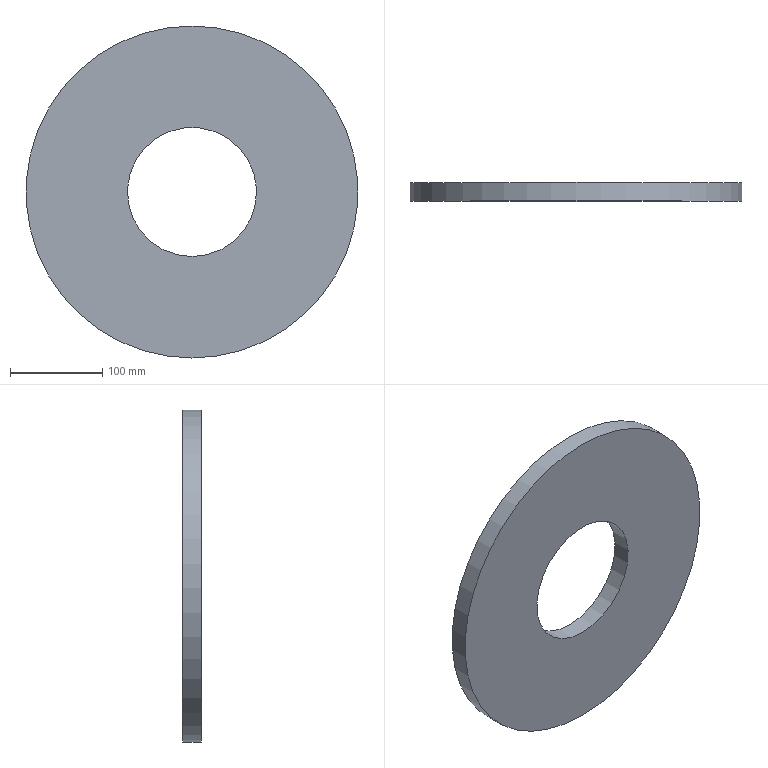Part | STEP file | 冲床-300配套压波_id730_x_t | 1 solid | 4 faces | box 360 x 20 x 360 mm | volume 1727876 mm3 | plane 2 | cylinder 2 | commonest cylinder face diameters 140 x1 360 x1
STEP:
#1=CARTESIAN_POINT('',(2195.,-10.,-275.));
#2=VERTEX_POINT('',#1);
#3=CARTESIAN_POINT('',(2195.,-10.,-205.));
#4=DIRECTION('',(0.,-1.,0.));
#5=DIRECTION('',(0.,0.,-1.));
#6=AXIS2_PLACEMENT_3D('',#3,#4,#5);
#7=CIRCLE('',#6,70.);
#8=EDGE_CURVE('',#2,#2,#7,.T.);
#9=ORIENTED_EDGE('',*,*,#8,.F.);
#10=EDGE_LOOP('',(#9));
#11=FACE_BOUND('',#10,.T.);
#12=CARTESIAN_POINT('',(2195.,-10.,-385.));
#13=VERTEX_POINT('',#12);
#14=CARTESIAN_POINT('',(2195.,-10.,-205.));
#15=DIRECTION('',(0.,-1.,0.));
#16=DIRECTION('',(0.,0.,-1.));
#17=AXIS2_PLACEMENT_3D('',#14,#15,#16);
#18=CIRCLE('',#17,180.);
#19=EDGE_CURVE('',#13,#13,#18,.T.);
#20=ORIENTED_EDGE('',*,*,#19,.T.);
#21=EDGE_LOOP('',(#20));
#22=FACE_BOUND('',#21,.T.);
#23=CARTESIAN_POINT('',(432.953,-10.,916.258));
#24=DIRECTION('',(0.,-1.,0.));
#25=DIRECTION('',(-0.5361,0.,-0.8442));
#26=AXIS2_PLACEMENT_3D('',#23,#24,#25);
#27=PLANE('',#26);
#28=ADVANCED_FACE('',(#11,#22),#27,.T.);
#29=CARTESIAN_POINT('',(2195.,10.,-275.));
#30=VERTEX_POINT('',#29);
#31=CARTESIAN_POINT('',(2195.,10.,-205.));
#32=DIRECTION('',(0.,-1.,0.));
#33=DIRECTION('',(0.,0.,-1.));
#34=AXIS2_PLACEMENT_3D('',#31,#32,#33);
#35=CIRCLE('',#34,70.);
#36=EDGE_CURVE('',#30,#30,#35,.T.);
#37=ORIENTED_EDGE('',*,*,#36,.T.);
#38=EDGE_LOOP('',(#37));
#39=FACE_BOUND('',#38,.T.);
#40=CARTESIAN_POINT('',(2195.,10.,-385.));
#41=VERTEX_POINT('',#40);
#42=CARTESIAN_POINT('',(2195.,10.,-205.));
#43=DIRECTION('',(0.,-1.,0.));
#44=DIRECTION('',(0.,0.,-1.));
#45=AXIS2_PLACEMENT_3D('',#42,#43,#44);
#46=CIRCLE('',#45,180.);
#47=EDGE_CURVE('',#41,#41,#46,.T.);
#48=ORIENTED_EDGE('',*,*,#47,.F.);
#49=EDGE_LOOP('',(#48));
#50=FACE_BOUND('',#49,.T.);
#51=CARTESIAN_POINT('',(432.953,10.,916.258));
#52=DIRECTION('',(0.,-1.,0.));
#53=DIRECTION('',(-0.5361,0.,-0.8442));
#54=AXIS2_PLACEMENT_3D('',#51,#52,#53);
#55=PLANE('',#54);
#56=ADVANCED_FACE('',(#39,#50),#55,.F.);
#57=ORIENTED_EDGE('',*,*,#8,.T.);
#58=EDGE_LOOP('',(#57));
#59=FACE_BOUND('',#58,.T.);
#60=ORIENTED_EDGE('',*,*,#36,.F.);
#61=EDGE_LOOP('',(#60));
#62=FACE_BOUND('',#61,.T.);
#63=CARTESIAN_POINT('',(2195.,-71.,-205.));
#64=DIRECTION('',(0.,1.,0.));
#65=DIRECTION('',(0.,0.,1.));
#66=AXIS2_PLACEMENT_3D('',#63,#64,#65);
#67=CYLINDRICAL_SURFACE('',#66,70.);
#68=ADVANCED_FACE('',(#59,#62),#67,.F.);
#69=ORIENTED_EDGE('',*,*,#19,.F.);
#70=EDGE_LOOP('',(#69));
#71=FACE_BOUND('',#70,.T.);
#72=ORIENTED_EDGE('',*,*,#47,.T.);
#73=EDGE_LOOP('',(#72));
#74=FACE_BOUND('',#73,.T.);
#75=CARTESIAN_POINT('',(2195.,-41.5,-205.));
#76=DIRECTION('',(0.,1.,0.));
#77=DIRECTION('',(0.,0.,1.));
#78=AXIS2_PLACEMENT_3D('',#75,#76,#77);
#79=CYLINDRICAL_SURFACE('',#78,180.);
#80=ADVANCED_FACE('',(#71,#74),#79,.T.);
#81=CLOSED_SHELL('',(#28,#56,#68,#80));
#82=MANIFOLD_SOLID_BREP('',#81);
#83=(LENGTH_UNIT()NAMED_UNIT(*)SI_UNIT(.MILLI.,.METRE.));
#84=UNCERTAINTY_MEASURE_WITH_UNIT(LENGTH_MEASURE(0.00002),#83,'','');
#85=(NAMED_UNIT(*)PLANE_ANGLE_UNIT()SI_UNIT($,.RADIAN.));
#86=PLANE_ANGLE_MEASURE_WITH_UNIT(PLANE_ANGLE_MEASURE(0.01745),#85);
#87=DIMENSIONAL_EXPONENTS(0.,0.,0.,0.,0.,0.,0.);
#88=(CONVERSION_BASED_UNIT('DEGREE',#86)NAMED_UNIT(#87)PLANE_ANGLE_UNIT());
#89=(NAMED_UNIT(*)SI_UNIT($,.STERADIAN.)SOLID_ANGLE_UNIT());
#90=(GEOMETRIC_REPRESENTATION_CONTEXT(3)GLOBAL_UNCERTAINTY_ASSIGNED_CONTEXT((#84))GLOBAL_UNIT_ASSIGNED_CONTEXT((#83,#88,#89))REPRESENTATION_CONTEXT('',''));
#91=ADVANCED_BREP_SHAPE_REPRESENTATION('',(#82),#90);